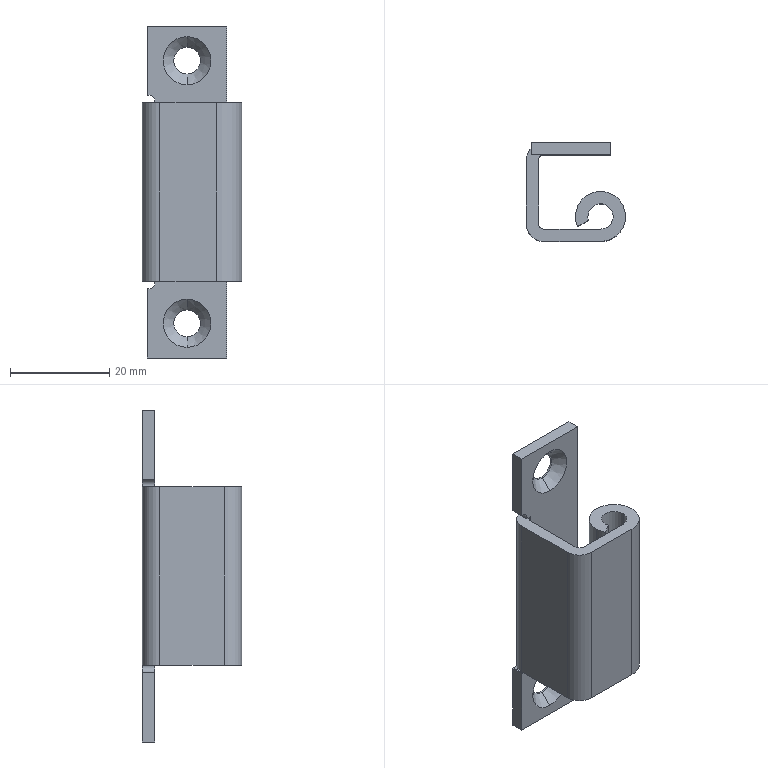Part | SolidWorks | features BaseBody 1 | 1 solid | 38 faces | box 20 x 20 x 67 mm | volume 6811 mm3 | plane 18 | cylinder 16 | cone 4 | commonest cylinder face diameters 5.4 x4 5.1 x3 10.1 x3 2 x2 2.5 x2 7 x2
STEP:
#1=CARTESIAN_POINT('',(-5.95,14.6,23.8));
#2=VERTEX_POINT('',#1);
#3=CARTESIAN_POINT('',(-5.95,14.6,29.2));
#4=VERTEX_POINT('',#3);
#5=CARTESIAN_POINT('',(-5.95,14.6,26.5));
#6=DIRECTION('',(0.,1.,0.));
#7=DIRECTION('',(0.,0.,1.));
#8=AXIS2_PLACEMENT_3D('',#5,#6,#7);
#9=CIRCLE('',#8,2.7);
#10=EDGE_CURVE('',#2,#4,#9,.T.);
#11=ORIENTED_EDGE('',*,*,#10,.F.);
#12=CARTESIAN_POINT('',(-5.95,14.95,23.8));
#13=VERTEX_POINT('',#12);
#14=CARTESIAN_POINT('',(-5.95,12.45,23.8));
#15=DIRECTION('',(0.,1.,0.));
#16=VECTOR('',#15,1000.);
#17=LINE('',#14,#16);
#18=EDGE_CURVE('',#2,#13,#17,.T.);
#19=ORIENTED_EDGE('',*,*,#18,.T.);
#20=CARTESIAN_POINT('',(-5.95,14.95,29.2));
#21=VERTEX_POINT('',#20);
#22=CARTESIAN_POINT('',(-5.95,14.95,26.5));
#23=DIRECTION('',(0.,1.,0.));
#24=DIRECTION('',(0.,0.,1.));
#25=AXIS2_PLACEMENT_3D('',#22,#23,#24);
#26=CIRCLE('',#25,2.7);
#27=EDGE_CURVE('',#13,#21,#26,.T.);
#28=ORIENTED_EDGE('',*,*,#27,.T.);
#29=CARTESIAN_POINT('',(-5.95,12.45,29.2));
#30=DIRECTION('',(0.,1.,0.));
#31=VECTOR('',#30,1000.);
#32=LINE('',#29,#31);
#33=EDGE_CURVE('',#4,#21,#32,.T.);
#34=ORIENTED_EDGE('',*,*,#33,.F.);
#35=EDGE_LOOP('',(#11,#19,#28,#34));
#36=FACE_OUTER_BOUND('',#35,.T.);
#37=CARTESIAN_POINT('',(-5.95,12.45,26.5));
#38=DIRECTION('',(0.,1.,0.));
#39=DIRECTION('',(0.,0.,1.));
#40=AXIS2_PLACEMENT_3D('',#37,#38,#39);
#41=CYLINDRICAL_SURFACE('',#40,2.7);
#42=ADVANCED_FACE('',(#36),#41,.F.);
#43=CARTESIAN_POINT('',(-5.95,14.6,-29.2));
#44=VERTEX_POINT('',#43);
#45=CARTESIAN_POINT('',(-5.95,14.6,-23.8));
#46=VERTEX_POINT('',#45);
#47=CARTESIAN_POINT('',(-5.95,14.6,-26.5));
#48=DIRECTION('',(0.,1.,0.));
#49=DIRECTION('',(0.,0.,1.));
#50=AXIS2_PLACEMENT_3D('',#47,#48,#49);
#51=CIRCLE('',#50,2.7);
#52=EDGE_CURVE('',#44,#46,#51,.T.);
#53=ORIENTED_EDGE('',*,*,#52,.F.);
#54=CARTESIAN_POINT('',(-5.95,14.95,-29.2));
#55=VERTEX_POINT('',#54);
#56=CARTESIAN_POINT('',(-5.95,12.45,-29.2));
#57=DIRECTION('',(0.,1.,0.));
#58=VECTOR('',#57,1000.);
#59=LINE('',#56,#58);
#60=EDGE_CURVE('',#44,#55,#59,.T.);
#61=ORIENTED_EDGE('',*,*,#60,.T.);
#62=CARTESIAN_POINT('',(-5.95,14.95,-23.8));
#63=VERTEX_POINT('',#62);
#64=CARTESIAN_POINT('',(-5.95,14.95,-26.5));
#65=DIRECTION('',(0.,1.,0.));
#66=DIRECTION('',(0.,0.,1.));
#67=AXIS2_PLACEMENT_3D('',#64,#65,#66);
#68=CIRCLE('',#67,2.7);
#69=EDGE_CURVE('',#55,#63,#68,.T.);
#70=ORIENTED_EDGE('',*,*,#69,.T.);
#71=CARTESIAN_POINT('',(-5.95,12.45,-23.8));
#72=DIRECTION('',(0.,1.,0.));
#73=VECTOR('',#72,1000.);
#74=LINE('',#71,#73);
#75=EDGE_CURVE('',#46,#63,#74,.T.);
#76=ORIENTED_EDGE('',*,*,#75,.F.);
#77=EDGE_LOOP('',(#53,#61,#70,#76));
#78=FACE_OUTER_BOUND('',#77,.T.);
#79=CARTESIAN_POINT('',(-5.95,12.45,-26.5));
#80=DIRECTION('',(0.,1.,0.));
#81=DIRECTION('',(0.,0.,1.));
#82=AXIS2_PLACEMENT_3D('',#79,#80,#81);
#83=CYLINDRICAL_SURFACE('',#82,2.7);
#84=ADVANCED_FACE('',(#78),#83,.F.);
#85=ORIENTED_EDGE('',*,*,#10,.T.);
#86=CARTESIAN_POINT('',(-5.95,12.45,31.35));
#87=VERTEX_POINT('',#86);
#88=CARTESIAN_POINT('',(-5.95,12.45,31.35));
#89=DIRECTION('',(0.,-0.7071,0.7071));
#90=VECTOR('',#89,1000.);
#91=LINE('',#88,#90);
#92=EDGE_CURVE('',#4,#87,#91,.T.);
#93=ORIENTED_EDGE('',*,*,#92,.T.);
#94=CARTESIAN_POINT('',(-5.95,12.45,21.65));
#95=VERTEX_POINT('',#94);
#96=CARTESIAN_POINT('',(-5.95,12.45,26.5));
#97=DIRECTION('',(0.,-1.,0.));
#98=DIRECTION('',(0.,0.,-1.));
#99=AXIS2_PLACEMENT_3D('',#96,#97,#98);
#100=CIRCLE('',#99,4.85);
#101=EDGE_CURVE('',#87,#95,#100,.T.);
#102=ORIENTED_EDGE('',*,*,#101,.T.);
#103=CARTESIAN_POINT('',(-5.95,12.45,21.65));
#104=DIRECTION('',(0.,-0.7071,-0.7071));
#105=VECTOR('',#104,1000.);
#106=LINE('',#103,#105);
#107=EDGE_CURVE('',#2,#95,#106,.T.);
#108=ORIENTED_EDGE('',*,*,#107,.F.);
#109=EDGE_LOOP('',(#85,#93,#102,#108));
#110=FACE_OUTER_BOUND('',#109,.T.);
#111=CARTESIAN_POINT('',(-5.95,12.45,26.5));
#112=DIRECTION('',(0.,-1.,0.));
#113=DIRECTION('',(0.,0.,-1.));
#114=AXIS2_PLACEMENT_3D('',#111,#112,#113);
#115=CONICAL_SURFACE('',#114,4.85,0.7854);
#116=ADVANCED_FACE('',(#110),#115,.F.);
#117=ORIENTED_EDGE('',*,*,#52,.T.);
#118=CARTESIAN_POINT('',(-5.95,12.45,-21.65));
#119=VERTEX_POINT('',#118);
#120=CARTESIAN_POINT('',(-5.95,12.45,-21.65));
#121=DIRECTION('',(0.,-0.7071,0.7071));
#122=VECTOR('',#121,1000.);
#123=LINE('',#120,#122);
#124=EDGE_CURVE('',#46,#119,#123,.T.);
#125=ORIENTED_EDGE('',*,*,#124,.T.);
#126=CARTESIAN_POINT('',(-5.95,12.45,-31.35));
#127=VERTEX_POINT('',#126);
#128=CARTESIAN_POINT('',(-5.95,12.45,-26.5));
#129=DIRECTION('',(0.,-1.,0.));
#130=DIRECTION('',(0.,0.,-1.));
#131=AXIS2_PLACEMENT_3D('',#128,#129,#130);
#132=CIRCLE('',#131,4.85);
#133=EDGE_CURVE('',#119,#127,#132,.T.);
#134=ORIENTED_EDGE('',*,*,#133,.T.);
#135=CARTESIAN_POINT('',(-5.95,12.45,-31.35));
#136=DIRECTION('',(0.,-0.7071,-0.7071));
#137=VECTOR('',#136,1000.);
#138=LINE('',#135,#137);
#139=EDGE_CURVE('',#44,#127,#138,.T.);
#140=ORIENTED_EDGE('',*,*,#139,.F.);
#141=EDGE_LOOP('',(#117,#125,#134,#140));
#142=FACE_OUTER_BOUND('',#141,.T.);
#143=CARTESIAN_POINT('',(-5.95,12.45,-26.5));
#144=DIRECTION('',(0.,-1.,0.));
#145=DIRECTION('',(0.,0.,-1.));
#146=AXIS2_PLACEMENT_3D('',#143,#144,#145);
#147=CONICAL_SURFACE('',#146,4.85,0.7854);
#148=ADVANCED_FACE('',(#142),#147,.F.);
#149=CARTESIAN_POINT('',(-2.426,-0.7856,-18.));
#150=VERTEX_POINT('',#149);
#151=CARTESIAN_POINT('',(-2.55,0.,-18.));
#152=VERTEX_POINT('',#151);
#153=CARTESIAN_POINT('',(0.,0.,-18.));
#154=DIRECTION('',(0.,0.,-1.));
#155=DIRECTION('',(1.,0.,0.));
#156=AXIS2_PLACEMENT_3D('',#153,#154,#155);
#157=CIRCLE('',#156,2.55);
#158=EDGE_CURVE('',#150,#152,#157,.T.);
#159=ORIENTED_EDGE('',*,*,#158,.T.);
#160=CARTESIAN_POINT('',(-2.55,0.,18.));
#161=VERTEX_POINT('',#160);
#162=CARTESIAN_POINT('',(-2.55,0.,18.));
#163=DIRECTION('',(0.,0.,1.));
#164=VECTOR('',#163,1000.);
#165=LINE('',#162,#164);
#166=EDGE_CURVE('',#152,#161,#165,.T.);
#167=ORIENTED_EDGE('',*,*,#166,.T.);
#168=CARTESIAN_POINT('',(-2.426,-0.7856,18.));
#169=VERTEX_POINT('',#168);
#170=CARTESIAN_POINT('',(0.,0.,18.));
#171=DIRECTION('',(0.,0.,-1.));
#172=DIRECTION('',(1.,0.,0.));
#173=AXIS2_PLACEMENT_3D('',#170,#171,#172);
#174=CIRCLE('',#173,2.55);
#175=EDGE_CURVE('',#169,#161,#174,.T.);
#176=ORIENTED_EDGE('',*,*,#175,.F.);
#177=CARTESIAN_POINT('',(-2.426,-0.7856,18.));
#178=DIRECTION('',(0.,0.,-1.));
#179=VECTOR('',#178,1000.);
#180=LINE('',#177,#179);
#181=EDGE_CURVE('',#169,#150,#180,.T.);
#182=ORIENTED_EDGE('',*,*,#181,.T.);
#183=EDGE_LOOP('',(#159,#167,#176,#182));
#184=FACE_OUTER_BOUND('',#183,.T.);
#185=CARTESIAN_POINT('',(0.,0.,18.));
#186=DIRECTION('',(0.,0.,1.));
#187=DIRECTION('',(1.,0.,0.));
#188=AXIS2_PLACEMENT_3D('',#185,#186,#187);
#189=CYLINDRICAL_SURFACE('',#188,2.55);
#190=ADVANCED_FACE('',(#184),#189,.F.);
#191=ORIENTED_EDGE('',*,*,#166,.F.);
#192=CARTESIAN_POINT('',(2.55,0.,-18.));
#193=VERTEX_POINT('',#192);
#194=CARTESIAN_POINT('',(0.,0.,-18.));
#195=DIRECTION('',(0.,0.,-1.));
#196=DIRECTION('',(1.,0.,0.));
#197=AXIS2_PLACEMENT_3D('',#194,#195,#196);
#198=CIRCLE('',#197,2.55);
#199=EDGE_CURVE('',#152,#193,#198,.T.);
#200=ORIENTED_EDGE('',*,*,#199,.T.);
#201=CARTESIAN_POINT('',(2.55,0.,18.));
#202=VERTEX_POINT('',#201);
#203=CARTESIAN_POINT('',(2.55,0.,18.));
#204=DIRECTION('',(0.,0.,1.));
#205=VECTOR('',#204,1000.);
#206=LINE('',#203,#205);
#207=EDGE_CURVE('',#193,#202,#206,.T.);
#208=ORIENTED_EDGE('',*,*,#207,.T.);
#209=CARTESIAN_POINT('',(0.,0.,18.));
#210=DIRECTION('',(0.,0.,-1.));
#211=DIRECTION('',(1.,0.,0.));
#212=AXIS2_PLACEMENT_3D('',#209,#210,#211);
#213=CIRCLE('',#212,2.55);
#214=EDGE_CURVE('',#161,#202,#213,.T.);
#215=ORIENTED_EDGE('',*,*,#214,.F.);
#216=EDGE_LOOP('',(#191,#200,#208,#215));
#217=FACE_OUTER_BOUND('',#216,.T.);
#218=CARTESIAN_POINT('',(0.,0.,18.));
#219=DIRECTION('',(0.,0.,1.));
#220=DIRECTION('',(1.,0.,0.));
#221=AXIS2_PLACEMENT_3D('',#218,#219,#220);
#222=CYLINDRICAL_SURFACE('',#221,2.55);
#223=ADVANCED_FACE('',(#217),#222,.F.);
#224=CARTESIAN_POINT('',(5.05,0.,-18.));
#225=VERTEX_POINT('',#224);
#226=CARTESIAN_POINT('',(-5.05,0.,-18.));
#227=VERTEX_POINT('',#226);
#228=CARTESIAN_POINT('',(0.,0.,-18.));
#229=DIRECTION('',(0.,0.,1.));
#230=DIRECTION('',(1.,0.,0.));
#231=AXIS2_PLACEMENT_3D('',#228,#229,#230);
#232=CIRCLE('',#231,5.05);
#233=EDGE_CURVE('',#225,#227,#232,.T.);
#234=ORIENTED_EDGE('',*,*,#233,.T.);
#235=CARTESIAN_POINT('',(-5.05,0.,18.));
#236=VERTEX_POINT('',#235);
#237=CARTESIAN_POINT('',(-5.05,0.,18.));
#238=DIRECTION('',(0.,0.,1.));
#239=VECTOR('',#238,1000.);
#240=LINE('',#237,#239);
#241=EDGE_CURVE('',#227,#236,#240,.T.);
#242=ORIENTED_EDGE('',*,*,#241,.T.);
#243=CARTESIAN_POINT('',(5.05,0.,18.));
#244=VERTEX_POINT('',#243);
#245=CARTESIAN_POINT('',(0.,0.,18.));
#246=DIRECTION('',(0.,0.,1.));
#247=DIRECTION('',(1.,0.,0.));
#248=AXIS2_PLACEMENT_3D('',#245,#246,#247);
#249=CIRCLE('',#248,5.05);
#250=EDGE_CURVE('',#244,#236,#249,.T.);
#251=ORIENTED_EDGE('',*,*,#250,.F.);
#252=CARTESIAN_POINT('',(5.05,0.,18.));
#253=DIRECTION('',(0.,0.,1.));
#254=VECTOR('',#253,1000.);
#255=LINE('',#252,#254);
#256=EDGE_CURVE('',#225,#244,#255,.T.);
#257=ORIENTED_EDGE('',*,*,#256,.F.);
#258=EDGE_LOOP('',(#234,#242,#251,#257));
#259=FACE_OUTER_BOUND('',#258,.T.);
#260=CARTESIAN_POINT('',(0.,0.,18.));
#261=DIRECTION('',(0.,0.,1.));
#262=DIRECTION('',(1.,0.,0.));
#263=AXIS2_PLACEMENT_3D('',#260,#261,#262);
#264=CYLINDRICAL_SURFACE('',#263,5.05);
#265=ADVANCED_FACE('',(#259),#264,.T.);
#266=CARTESIAN_POINT('',(0.,-5.05,-18.));
#267=VERTEX_POINT('',#266);
#268=CARTESIAN_POINT('',(0.,0.,-18.));
#269=DIRECTION('',(0.,0.,1.));
#270=DIRECTION('',(1.,0.,0.));
#271=AXIS2_PLACEMENT_3D('',#268,#269,#270);
#272=CIRCLE('',#271,5.05);
#273=EDGE_CURVE('',#267,#225,#272,.T.);
#274=ORIENTED_EDGE('',*,*,#273,.T.);
#275=ORIENTED_EDGE('',*,*,#256,.T.);
#276=CARTESIAN_POINT('',(0.,-5.05,18.));
#277=VERTEX_POINT('',#276);
#278=CARTESIAN_POINT('',(0.,0.,18.));
#279=DIRECTION('',(0.,0.,1.));
#280=DIRECTION('',(1.,0.,0.));
#281=AXIS2_PLACEMENT_3D('',#278,#279,#280);
#282=CIRCLE('',#281,5.05);
#283=EDGE_CURVE('',#277,#244,#282,.T.);
#284=ORIENTED_EDGE('',*,*,#283,.F.);
#285=CARTESIAN_POINT('',(0.,-5.05,18.));
#286=DIRECTION('',(0.,0.,-1.));
#287=VECTOR('',#286,1000.);
#288=LINE('',#285,#287);
#289=EDGE_CURVE('',#277,#267,#288,.T.);
#290=ORIENTED_EDGE('',*,*,#289,.T.);
#291=EDGE_LOOP('',(#274,#275,#284,#290));
#292=FACE_OUTER_BOUND('',#291,.T.);
#293=CARTESIAN_POINT('',(0.,0.,18.));
#294=DIRECTION('',(0.,0.,1.));
#295=DIRECTION('',(1.,0.,0.));
#296=AXIS2_PLACEMENT_3D('',#293,#294,#295);
#297=CYLINDRICAL_SURFACE('',#296,5.05);
#298=ADVANCED_FACE('',(#292),#297,.T.);
#299=CARTESIAN_POINT('',(-13.95,14.95,-33.5));
#300=VERTEX_POINT('',#299);
#301=CARTESIAN_POINT('',(2.05,14.95,-33.5));
#302=VERTEX_POINT('',#301);
#303=CARTESIAN_POINT('',(2.05,14.95,-33.5));
#304=DIRECTION('',(1.,0.,0.));
#305=VECTOR('',#304,1000.);
#306=LINE('',#303,#305);
#307=EDGE_CURVE('',#300,#302,#306,.T.);
#308=ORIENTED_EDGE('',*,*,#307,.F.);
#309=CARTESIAN_POINT('',(-13.95,14.95,-19.5));
#310=VERTEX_POINT('',#309);
#311=CARTESIAN_POINT('',(-13.95,14.95,18.));
#312=DIRECTION('',(0.,0.,-1.));
#313=VECTOR('',#312,1000.);
#314=LINE('',#311,#313);
#315=EDGE_CURVE('',#310,#300,#314,.T.);
#316=ORIENTED_EDGE('',*,*,#315,.F.);
#317=CARTESIAN_POINT('',(-13.675,14.95,-19.5));
#318=VERTEX_POINT('',#317);
#319=CARTESIAN_POINT('',(-13.95,14.95,-19.5));
#320=DIRECTION('',(-1.,0.,0.));
#321=VECTOR('',#320,1000.);
#322=LINE('',#319,#321);
#323=EDGE_CURVE('',#318,#310,#322,.T.);
#324=ORIENTED_EDGE('',*,*,#323,.F.);
#325=CARTESIAN_POINT('',(-12.45,14.95,-18.));
#326=VERTEX_POINT('',#325);
#327=CARTESIAN_POINT('',(-13.675,14.95,-18.25));
#328=DIRECTION('',(0.,1.,0.));
#329=DIRECTION('',(0.,0.,-1.));
#330=AXIS2_PLACEMENT_3D('',#327,#328,#329);
#331=CIRCLE('',#330,1.25);
#332=EDGE_CURVE('',#326,#318,#331,.T.);
#333=ORIENTED_EDGE('',*,*,#332,.F.);
#334=CARTESIAN_POINT('',(-11.45,14.95,-18.));
#335=VERTEX_POINT('',#334);
#336=CARTESIAN_POINT('',(2.05,14.95,-18.));
#337=DIRECTION('',(-1.,0.,0.));
#338=VECTOR('',#337,1000.);
#339=LINE('',#336,#338);
#340=EDGE_CURVE('',#335,#326,#339,.T.);
#341=ORIENTED_EDGE('',*,*,#340,.F.);
#342=CARTESIAN_POINT('',(-11.45,14.95,18.));
#343=VERTEX_POINT('',#342);
#344=CARTESIAN_POINT('',(-11.45,14.95,18.));
#345=DIRECTION('',(0.,0.,-1.));
#346=VECTOR('',#345,1000.);
#347=LINE('',#344,#346);
#348=EDGE_CURVE('',#343,#335,#347,.T.);
#349=ORIENTED_EDGE('',*,*,#348,.F.);
#350=CARTESIAN_POINT('',(-12.45,14.95,18.));
#351=VERTEX_POINT('',#350);
#352=CARTESIAN_POINT('',(2.05,14.95,18.));
#353=DIRECTION('',(1.,0.,0.));
#354=VECTOR('',#353,1000.);
#355=LINE('',#352,#354);
#356=EDGE_CURVE('',#351,#343,#355,.T.);
#357=ORIENTED_EDGE('',*,*,#356,.F.);
#358=CARTESIAN_POINT('',(-13.675,14.95,19.5));
#359=VERTEX_POINT('',#358);
#360=CARTESIAN_POINT('',(-13.675,14.95,18.25));
#361=DIRECTION('',(0.,1.,0.));
#362=DIRECTION('',(0.,0.,-1.));
#363=AXIS2_PLACEMENT_3D('',#360,#361,#362);
#364=CIRCLE('',#363,1.25);
#365=EDGE_CURVE('',#359,#351,#364,.T.);
#366=ORIENTED_EDGE('',*,*,#365,.F.);
#367=CARTESIAN_POINT('',(-13.95,14.95,19.5));
#368=VERTEX_POINT('',#367);
#369=CARTESIAN_POINT('',(-13.675,14.95,19.5));
#370=DIRECTION('',(1.,0.,0.));
#371=VECTOR('',#370,1000.);
#372=LINE('',#369,#371);
#373=EDGE_CURVE('',#368,#359,#372,.T.);
#374=ORIENTED_EDGE('',*,*,#373,.F.);
#375=CARTESIAN_POINT('',(-13.95,14.95,33.5));
#376=VERTEX_POINT('',#375);
#377=CARTESIAN_POINT('',(-13.95,14.95,18.));
#378=DIRECTION('',(0.,0.,-1.));
#379=VECTOR('',#378,1000.);
#380=LINE('',#377,#379);
#381=EDGE_CURVE('',#376,#368,#380,.T.);
#382=ORIENTED_EDGE('',*,*,#381,.F.);
#383=CARTESIAN_POINT('',(2.05,14.95,33.5));
#384=VERTEX_POINT('',#383);
#385=CARTESIAN_POINT('',(2.05,14.95,33.5));
#386=DIRECTION('',(-1.,0.,0.));
#387=VECTOR('',#386,1000.);
#388=LINE('',#385,#387);
#389=EDGE_CURVE('',#384,#376,#388,.T.);
#390=ORIENTED_EDGE('',*,*,#389,.F.);
#391=CARTESIAN_POINT('',(2.05,14.95,18.));
#392=DIRECTION('',(0.,0.,1.));
#393=VECTOR('',#392,1000.);
#394=LINE('',#391,#393);
#395=EDGE_CURVE('',#302,#384,#394,.T.);
#396=ORIENTED_EDGE('',*,*,#395,.F.);
#397=EDGE_LOOP('',(#308,#316,#324,#333,#341,#349,#357,#366,#374,#382,#390,#396));
#398=FACE_OUTER_BOUND('',#397,.T.);
#399=CARTESIAN_POINT('',(-5.95,14.95,26.5));
#400=DIRECTION('',(0.,1.,0.));
#401=DIRECTION('',(0.,0.,1.));
#402=AXIS2_PLACEMENT_3D('',#399,#400,#401);
#403=CIRCLE('',#402,2.7);
#404=EDGE_CURVE('',#21,#13,#403,.T.);
#405=ORIENTED_EDGE('',*,*,#404,.F.);
#406=ORIENTED_EDGE('',*,*,#27,.F.);
#407=EDGE_LOOP('',(#405,#406));
#408=FACE_BOUND('',#407,.T.);
#409=CARTESIAN_POINT('',(-5.95,14.95,-26.5));
#410=DIRECTION('',(0.,1.,0.));
#411=DIRECTION('',(0.,0.,1.));
#412=AXIS2_PLACEMENT_3D('',#409,#410,#411);
#413=CIRCLE('',#412,2.7);
#414=EDGE_CURVE('',#63,#55,#413,.T.);
#415=ORIENTED_EDGE('',*,*,#414,.F.);
#416=ORIENTED_EDGE('',*,*,#69,.F.);
#417=EDGE_LOOP('',(#415,#416));
#418=FACE_BOUND('',#417,.T.);
#419=CARTESIAN_POINT('',(2.05,14.95,18.));
#420=DIRECTION('',(0.,-1.,0.));
#421=DIRECTION('',(0.,0.,-1.));
#422=AXIS2_PLACEMENT_3D('',#419,#420,#421);
#423=PLANE('',#422);
#424=ADVANCED_FACE('',(#398,#408,#418),#423,.F.);
#425=CARTESIAN_POINT('',(2.05,12.45,-33.5));
#426=VERTEX_POINT('',#425);
#427=CARTESIAN_POINT('',(2.05,12.45,-33.5));
#428=DIRECTION('',(0.,-1.,0.));
#429=VECTOR('',#428,1000.);
#430=LINE('',#427,#429);
#431=EDGE_CURVE('',#302,#426,#430,.T.);
#432=ORIENTED_EDGE('',*,*,#431,.F.);
#433=ORIENTED_EDGE('',*,*,#395,.T.);
#434=CARTESIAN_POINT('',(2.05,12.45,33.5));
#435=VERTEX_POINT('',#434);
#436=CARTESIAN_POINT('',(2.05,12.45,33.5));
#437=DIRECTION('',(0.,1.,0.));
#438=VECTOR('',#437,1000.);
#439=LINE('',#436,#438);
#440=EDGE_CURVE('',#435,#384,#439,.T.);
#441=ORIENTED_EDGE('',*,*,#440,.F.);
#442=CARTESIAN_POINT('',(2.05,12.45,18.));
#443=DIRECTION('',(0.,0.,1.));
#444=VECTOR('',#443,1000.);
#445=LINE('',#442,#444);
#446=EDGE_CURVE('',#426,#435,#445,.T.);
#447=ORIENTED_EDGE('',*,*,#446,.F.);
#448=EDGE_LOOP('',(#432,#433,#441,#447));
#449=FACE_OUTER_BOUND('',#448,.T.);
#450=CARTESIAN_POINT('',(2.05,12.45,18.));
#451=DIRECTION('',(-1.,0.,0.));
#452=DIRECTION('',(0.,0.,1.));
#453=AXIS2_PLACEMENT_3D('',#450,#451,#452);
#454=PLANE('',#453);
#455=ADVANCED_FACE('',(#449),#454,.F.);
#456=CARTESIAN_POINT('',(-13.95,12.45,-33.5));
#457=VERTEX_POINT('',#456);
#458=CARTESIAN_POINT('',(2.05,12.45,-33.5));
#459=DIRECTION('',(-1.,0.,0.));
#460=VECTOR('',#459,1000.);
#461=LINE('',#458,#460);
#462=EDGE_CURVE('',#426,#457,#461,.T.);
#463=ORIENTED_EDGE('',*,*,#462,.T.);
#464=CARTESIAN_POINT('',(-13.95,12.45,-33.5));
#465=DIRECTION('',(0.,1.,0.));
#466=VECTOR('',#465,1000.);
#467=LINE('',#464,#466);
#468=EDGE_CURVE('',#457,#300,#467,.T.);
#469=ORIENTED_EDGE('',*,*,#468,.T.);
#470=ORIENTED_EDGE('',*,*,#307,.T.);
#471=ORIENTED_EDGE('',*,*,#431,.T.);
#472=EDGE_LOOP('',(#463,#469,#470,#471));
#473=FACE_OUTER_BOUND('',#472,.T.);
#474=CARTESIAN_POINT('',(2.05,12.45,-33.5));
#475=DIRECTION('',(0.,0.,-1.));
#476=DIRECTION('',(-1.,0.,0.));
#477=AXIS2_PLACEMENT_3D('',#474,#475,#476);
#478=PLANE('',#477);
#479=ADVANCED_FACE('',(#473),#478,.T.);
#480=CARTESIAN_POINT('',(-13.95,12.45,-19.5));
#481=VERTEX_POINT('',#480);
#482=CARTESIAN_POINT('',(-13.95,12.45,-33.5));
#483=DIRECTION('',(0.,0.,1.));
#484=VECTOR('',#483,1000.);
#485=LINE('',#482,#484);
#486=EDGE_CURVE('',#457,#481,#485,.T.);
#487=ORIENTED_EDGE('',*,*,#486,.T.);
#488=CARTESIAN_POINT('',(-13.95,12.45,-19.5));
#489=DIRECTION('',(0.,1.,0.));
#490=VECTOR('',#489,1000.);
#491=LINE('',#488,#490);
#492=EDGE_CURVE('',#481,#310,#491,.T.);
#493=ORIENTED_EDGE('',*,*,#492,.T.);
#494=ORIENTED_EDGE('',*,*,#315,.T.);
#495=ORIENTED_EDGE('',*,*,#468,.F.);
#496=EDGE_LOOP('',(#487,#493,#494,#495));
#497=FACE_OUTER_BOUND('',#496,.T.);
#498=CARTESIAN_POINT('',(-13.95,12.45,-33.5));
#499=DIRECTION('',(-1.,0.,0.));
#500=DIRECTION('',(0.,0.,1.));
#501=AXIS2_PLACEMENT_3D('',#498,#499,#500);
#502=PLANE('',#501);
#503=ADVANCED_FACE('',(#497),#502,.T.);
#504=ORIENTED_EDGE('',*,*,#332,.T.);
#505=CARTESIAN_POINT('',(-13.675,12.45,-19.5));
#506=VERTEX_POINT('',#505);
#507=CARTESIAN_POINT('',(-13.675,12.45,-19.5));
#508=DIRECTION('',(0.,1.,0.));
#509=VECTOR('',#508,1000.);
#510=LINE('',#507,#509);
#511=EDGE_CURVE('',#506,#318,#510,.T.);
#512=ORIENTED_EDGE('',*,*,#511,.F.);
#513=CARTESIAN_POINT('',(-12.45,12.45,-18.));
#514=VERTEX_POINT('',#513);
#515=CARTESIAN_POINT('',(-13.675,12.45,-18.25));
#516=DIRECTION('',(0.,1.,0.));
#517=DIRECTION('',(0.,0.,-1.));
#518=AXIS2_PLACEMENT_3D('',#515,#516,#517);
#519=CIRCLE('',#518,1.25);
#520=EDGE_CURVE('',#514,#506,#519,.T.);
#521=ORIENTED_EDGE('',*,*,#520,.F.);
#522=CARTESIAN_POINT('',(-12.45,14.804,-18.));
#523=VERTEX_POINT('',#522);
#524=CARTESIAN_POINT('',(-12.45,12.45,-18.));
#525=DIRECTION('',(0.,-1.,0.));
#526=VECTOR('',#525,1000.);
#527=LINE('',#524,#526);
#528=EDGE_CURVE('',#523,#514,#527,.T.);
#529=ORIENTED_EDGE('',*,*,#528,.F.);
#530=CARTESIAN_POINT('',(-12.45,12.45,-18.));
#531=DIRECTION('',(0.,-1.,0.));
#532=VECTOR('',#531,1000.);
#533=LINE('',#530,#532);
#534=EDGE_CURVE('',#326,#523,#533,.T.);
#535=ORIENTED_EDGE('',*,*,#534,.F.);
#536=EDGE_LOOP('',(#504,#512,#521,#529,#535));
#537=FACE_OUTER_BOUND('',#536,.T.);
#538=CARTESIAN_POINT('',(-13.675,12.45,-18.25));
#539=DIRECTION('',(0.,-1.,0.));
#540=DIRECTION('',(0.,0.,-1.));
#541=AXIS2_PLACEMENT_3D('',#538,#539,#540);
#542=CYLINDRICAL_SURFACE('',#541,1.25);
#543=ADVANCED_FACE('',(#537),#542,.F.);
#544=ORIENTED_EDGE('',*,*,#340,.T.);
#545=ORIENTED_EDGE('',*,*,#534,.T.);
#546=CARTESIAN_POINT('',(-11.45,11.45,-18.));
#547=DIRECTION('',(0.,0.,-1.));
#548=DIRECTION('',(1.,0.,0.));
#549=AXIS2_PLACEMENT_3D('',#546,#547,#548);
#550=CIRCLE('',#549,3.5);
#551=EDGE_CURVE('',#523,#335,#550,.T.);
#552=ORIENTED_EDGE('',*,*,#551,.T.);
#553=EDGE_LOOP('',(#544,#545,#552));
#554=FACE_OUTER_BOUND('',#553,.T.);
#555=CARTESIAN_POINT('',(-12.45,12.45,-18.));
#556=DIRECTION('',(0.,0.,1.));
#557=DIRECTION('',(1.,0.,0.));
#558=AXIS2_PLACEMENT_3D('',#555,#556,#557);
#559=PLANE('',#558);
#560=ADVANCED_FACE('',(#554),#559,.T.);
#561=CARTESIAN_POINT('',(-12.45,14.804,18.));
#562=VERTEX_POINT('',#561);
#563=CARTESIAN_POINT('',(-11.45,11.45,18.));
#564=DIRECTION('',(0.,0.,-1.));
#565=DIRECTION('',(1.,0.,0.));
#566=AXIS2_PLACEMENT_3D('',#563,#564,#565);
#567=CIRCLE('',#566,3.5);
#568=EDGE_CURVE('',#562,#343,#567,.T.);
#569=ORIENTED_EDGE('',*,*,#568,.T.);
#570=ORIENTED_EDGE('',*,*,#348,.T.);
#571=ORIENTED_EDGE('',*,*,#551,.F.);
#572=CARTESIAN_POINT('',(-14.95,11.45,-18.));
#573=VERTEX_POINT('',#572);
#574=CARTESIAN_POINT('',(-11.45,11.45,-18.));
#575=DIRECTION('',(0.,0.,1.));
#576=DIRECTION('',(1.,0.,0.));
#577=AXIS2_PLACEMENT_3D('',#574,#575,#576);
#578=CIRCLE('',#577,3.5);
#579=EDGE_CURVE('',#523,#573,#578,.T.);
#580=ORIENTED_EDGE('',*,*,#579,.T.);
#581=CARTESIAN_POINT('',(-14.95,11.45,18.));
#582=VERTEX_POINT('',#581);
#583=CARTESIAN_POINT('',(-14.95,11.45,18.));
#584=DIRECTION('',(0.,0.,1.));
#585=VECTOR('',#584,1000.);
#586=LINE('',#583,#585);
#587=EDGE_CURVE('',#573,#582,#586,.T.);
#588=ORIENTED_EDGE('',*,*,#587,.T.);
#589=CARTESIAN_POINT('',(-11.45,11.45,18.));
#590=DIRECTION('',(0.,0.,-1.));
#591=DIRECTION('',(1.,0.,0.));
#592=AXIS2_PLACEMENT_3D('',#589,#590,#591);
#593=CIRCLE('',#592,3.5);
#594=EDGE_CURVE('',#582,#562,#593,.T.);
#595=ORIENTED_EDGE('',*,*,#594,.T.);
#596=EDGE_LOOP('',(#569,#570,#571,#580,#588,#595));
#597=FACE_OUTER_BOUND('',#596,.T.);
#598=CARTESIAN_POINT('',(-11.45,11.45,18.));
#599=DIRECTION('',(0.,0.,1.));
#600=DIRECTION('',(1.,0.,0.));
#601=AXIS2_PLACEMENT_3D('',#598,#599,#600);
#602=CYLINDRICAL_SURFACE('',#601,3.5);
#603=ADVANCED_FACE('',(#597),#602,.T.);
#604=CARTESIAN_POINT('',(-12.45,12.45,18.));
#605=DIRECTION('',(0.,1.,0.));
#606=VECTOR('',#605,1000.);
#607=LINE('',#604,#606);
#608=EDGE_CURVE('',#562,#351,#607,.T.);
#609=ORIENTED_EDGE('',*,*,#608,.T.);
#610=ORIENTED_EDGE('',*,*,#356,.T.);
#611=ORIENTED_EDGE('',*,*,#568,.F.);
#612=EDGE_LOOP('',(#609,#610,#611));
#613=FACE_OUTER_BOUND('',#612,.T.);
#614=CARTESIAN_POINT('',(-11.45,12.45,18.));
#615=DIRECTION('',(0.,0.,-1.));
#616=DIRECTION('',(-1.,0.,0.));
#617=AXIS2_PLACEMENT_3D('',#614,#615,#616);
#618=PLANE('',#617);
#619=ADVANCED_FACE('',(#613),#618,.T.);
#620=ORIENTED_EDGE('',*,*,#365,.T.);
#621=ORIENTED_EDGE('',*,*,#608,.F.);
#622=CARTESIAN_POINT('',(-12.45,12.45,18.));
#623=VERTEX_POINT('',#622);
#624=CARTESIAN_POINT('',(-12.45,12.45,18.));
#625=DIRECTION('',(0.,1.,0.));
#626=VECTOR('',#625,1000.);
#627=LINE('',#624,#626);
#628=EDGE_CURVE('',#623,#562,#627,.T.);
#629=ORIENTED_EDGE('',*,*,#628,.F.);
#630=CARTESIAN_POINT('',(-13.675,12.45,19.5));
#631=VERTEX_POINT('',#630);
#632=CARTESIAN_POINT('',(-13.675,12.45,18.25));
#633=DIRECTION('',(0.,1.,0.));
#634=DIRECTION('',(0.,0.,-1.));
#635=AXIS2_PLACEMENT_3D('',#632,#633,#634);
#636=CIRCLE('',#635,1.25);
#637=EDGE_CURVE('',#631,#623,#636,.T.);
#638=ORIENTED_EDGE('',*,*,#637,.F.);
#639=CARTESIAN_POINT('',(-13.675,12.45,19.5));
#640=DIRECTION('',(0.,-1.,0.));
#641=VECTOR('',#640,1000.);
#642=LINE('',#639,#641);
#643=EDGE_CURVE('',#359,#631,#642,.T.);
#644=ORIENTED_EDGE('',*,*,#643,.F.);
#645=EDGE_LOOP('',(#620,#621,#629,#638,#644));
#646=FACE_OUTER_BOUND('',#645,.T.);
#647=CARTESIAN_POINT('',(-13.675,12.45,18.25));
#648=DIRECTION('',(0.,-1.,0.));
#649=DIRECTION('',(0.,0.,-1.));
#650=AXIS2_PLACEMENT_3D('',#647,#648,#649);
#651=CYLINDRICAL_SURFACE('',#650,1.25);
#652=ADVANCED_FACE('',(#646),#651,.F.);
#653=CARTESIAN_POINT('',(-13.95,12.45,19.5));
#654=VERTEX_POINT('',#653);
#655=CARTESIAN_POINT('',(-13.95,12.45,33.5));
#656=VERTEX_POINT('',#655);
#657=CARTESIAN_POINT('',(-13.95,12.45,19.5));
#658=DIRECTION('',(0.,0.,1.));
#659=VECTOR('',#658,1000.);
#660=LINE('',#657,#659);
#661=EDGE_CURVE('',#654,#656,#660,.T.);
#662=ORIENTED_EDGE('',*,*,#661,.T.);
#663=CARTESIAN_POINT('',(-13.95,12.45,33.5));
#664=DIRECTION('',(0.,1.,0.));
#665=VECTOR('',#664,1000.);
#666=LINE('',#663,#665);
#667=EDGE_CURVE('',#656,#376,#666,.T.);
#668=ORIENTED_EDGE('',*,*,#667,.T.);
#669=ORIENTED_EDGE('',*,*,#381,.T.);
#670=CARTESIAN_POINT('',(-13.95,12.45,19.5));
#671=DIRECTION('',(0.,-1.,0.));
#672=VECTOR('',#671,1000.);
#673=LINE('',#670,#672);
#674=EDGE_CURVE('',#368,#654,#673,.T.);
#675=ORIENTED_EDGE('',*,*,#674,.T.);
#676=EDGE_LOOP('',(#662,#668,#669,#675));
#677=FACE_OUTER_BOUND('',#676,.T.);
#678=CARTESIAN_POINT('',(-13.95,12.45,19.5));
#679=DIRECTION('',(-1.,0.,0.));
#680=DIRECTION('',(0.,0.,1.));
#681=AXIS2_PLACEMENT_3D('',#678,#679,#680);
#682=PLANE('',#681);
#683=ADVANCED_FACE('',(#677),#682,.T.);
#684=CARTESIAN_POINT('',(-13.95,12.45,33.5));
#685=DIRECTION('',(1.,0.,0.));
#686=VECTOR('',#685,1000.);
#687=LINE('',#684,#686);
#688=EDGE_CURVE('',#656,#435,#687,.T.);
#689=ORIENTED_EDGE('',*,*,#688,.T.);
#690=ORIENTED_EDGE('',*,*,#440,.T.);
#691=ORIENTED_EDGE('',*,*,#389,.T.);
#692=ORIENTED_EDGE('',*,*,#667,.F.);
#693=EDGE_LOOP('',(#689,#690,#691,#692));
#694=FACE_OUTER_BOUND('',#693,.T.);
#695=CARTESIAN_POINT('',(-13.95,12.45,33.5));
#696=DIRECTION('',(0.,0.,1.));
#697=DIRECTION('',(1.,0.,0.));
#698=AXIS2_PLACEMENT_3D('',#695,#696,#697);
#699=PLANE('',#698);
#700=ADVANCED_FACE('',(#694),#699,.T.);
#701=ORIENTED_EDGE('',*,*,#18,.F.);
#702=CARTESIAN_POINT('',(-5.95,14.6,26.5));
#703=DIRECTION('',(0.,1.,0.));
#704=DIRECTION('',(0.,0.,1.));
#705=AXIS2_PLACEMENT_3D('',#702,#703,#704);
#706=CIRCLE('',#705,2.7);
#707=EDGE_CURVE('',#4,#2,#706,.T.);
#708=ORIENTED_EDGE('',*,*,#707,.F.);
#709=ORIENTED_EDGE('',*,*,#33,.T.);
#710=ORIENTED_EDGE('',*,*,#404,.T.);
#711=EDGE_LOOP('',(#701,#708,#709,#710));
#712=FACE_OUTER_BOUND('',#711,.T.);
#713=CARTESIAN_POINT('',(-5.95,12.45,26.5));
#714=DIRECTION('',(0.,1.,0.));
#715=DIRECTION('',(0.,0.,1.));
#716=AXIS2_PLACEMENT_3D('',#713,#714,#715);
#717=CYLINDRICAL_SURFACE('',#716,2.7);
#718=ADVANCED_FACE('',(#712),#717,.F.);
#719=ORIENTED_EDGE('',*,*,#60,.F.);
#720=CARTESIAN_POINT('',(-5.95,14.6,-26.5));
#721=DIRECTION('',(0.,1.,0.));
#722=DIRECTION('',(0.,0.,1.));
#723=AXIS2_PLACEMENT_3D('',#720,#721,#722);
#724=CIRCLE('',#723,2.7);
#725=EDGE_CURVE('',#46,#44,#724,.T.);
#726=ORIENTED_EDGE('',*,*,#725,.F.);
#727=ORIENTED_EDGE('',*,*,#75,.T.);
#728=ORIENTED_EDGE('',*,*,#414,.T.);
#729=EDGE_LOOP('',(#719,#726,#727,#728));
#730=FACE_OUTER_BOUND('',#729,.T.);
#731=CARTESIAN_POINT('',(-5.95,12.45,-26.5));
#732=DIRECTION('',(0.,1.,0.));
#733=DIRECTION('',(0.,0.,1.));
#734=AXIS2_PLACEMENT_3D('',#731,#732,#733);
#735=CYLINDRICAL_SURFACE('',#734,2.7);
#736=ADVANCED_FACE('',(#730),#735,.F.);
#737=CARTESIAN_POINT('',(-11.45,12.45,-18.));
#738=VERTEX_POINT('',#737);
#739=CARTESIAN_POINT('',(-11.45,12.45,-18.));
#740=DIRECTION('',(1.,0.,0.));
#741=VECTOR('',#740,1000.);
#742=LINE('',#739,#741);
#743=EDGE_CURVE('',#514,#738,#742,.T.);
#744=ORIENTED_EDGE('',*,*,#743,.F.);
#745=ORIENTED_EDGE('',*,*,#520,.T.);
#746=CARTESIAN_POINT('',(-11.45,12.45,-19.5));
#747=DIRECTION('',(1.,0.,0.));
#748=VECTOR('',#747,1000.);
#749=LINE('',#746,#748);
#750=EDGE_CURVE('',#481,#506,#749,.T.);
#751=ORIENTED_EDGE('',*,*,#750,.F.);
#752=ORIENTED_EDGE('',*,*,#486,.F.);
#753=ORIENTED_EDGE('',*,*,#462,.F.);
#754=ORIENTED_EDGE('',*,*,#446,.T.);
#755=ORIENTED_EDGE('',*,*,#688,.F.);
#756=ORIENTED_EDGE('',*,*,#661,.F.);
#757=CARTESIAN_POINT('',(-11.45,12.45,19.5));
#758=DIRECTION('',(-1.,0.,0.));
#759=VECTOR('',#758,1000.);
#760=LINE('',#757,#759);
#761=EDGE_CURVE('',#631,#654,#760,.T.);
#762=ORIENTED_EDGE('',*,*,#761,.F.);
#763=ORIENTED_EDGE('',*,*,#637,.T.);
#764=CARTESIAN_POINT('',(-11.45,12.45,18.));
#765=VERTEX_POINT('',#764);
#766=CARTESIAN_POINT('',(-11.45,12.45,18.));
#767=DIRECTION('',(-1.,0.,0.));
#768=VECTOR('',#767,1000.);
#769=LINE('',#766,#768);
#770=EDGE_CURVE('',#765,#623,#769,.T.);
#771=ORIENTED_EDGE('',*,*,#770,.F.);
#772=CARTESIAN_POINT('',(-11.45,12.45,18.));
#773=DIRECTION('',(0.,0.,1.));
#774=VECTOR('',#773,1000.);
#775=LINE('',#772,#774);
#776=EDGE_CURVE('',#738,#765,#775,.T.);
#777=ORIENTED_EDGE('',*,*,#776,.F.);
#778=EDGE_LOOP('',(#744,#745,#751,#752,#753,#754,#755,#756,#762,#763,#771,#777));
#779=FACE_OUTER_BOUND('',#778,.T.);
#780=CARTESIAN_POINT('',(-5.95,12.45,26.5));
#781=DIRECTION('',(0.,-1.,0.));
#782=DIRECTION('',(0.,0.,-1.));
#783=AXIS2_PLACEMENT_3D('',#780,#781,#782);
#784=CIRCLE('',#783,4.85);
#785=EDGE_CURVE('',#95,#87,#784,.T.);
#786=ORIENTED_EDGE('',*,*,#785,.F.);
#787=ORIENTED_EDGE('',*,*,#101,.F.);
#788=EDGE_LOOP('',(#786,#787));
#789=FACE_BOUND('',#788,.T.);
#790=CARTESIAN_POINT('',(-5.95,12.45,-26.5));
#791=DIRECTION('',(0.,-1.,0.));
#792=DIRECTION('',(0.,0.,-1.));
#793=AXIS2_PLACEMENT_3D('',#790,#791,#792);
#794=CIRCLE('',#793,4.85);
#795=EDGE_CURVE('',#127,#119,#794,.T.);
#796=ORIENTED_EDGE('',*,*,#795,.F.);
#797=ORIENTED_EDGE('',*,*,#133,.F.);
#798=EDGE_LOOP('',(#796,#797));
#799=FACE_BOUND('',#798,.T.);
#800=CARTESIAN_POINT('',(-11.45,12.45,18.));
#801=DIRECTION('',(0.,1.,0.));
#802=DIRECTION('',(0.,0.,1.));
#803=AXIS2_PLACEMENT_3D('',#800,#801,#802);
#804=PLANE('',#803);
#805=ADVANCED_FACE('',(#779,#789,#799),#804,.F.);
#806=ORIENTED_EDGE('',*,*,#750,.T.);
#807=ORIENTED_EDGE('',*,*,#511,.T.);
#808=ORIENTED_EDGE('',*,*,#323,.T.);
#809=ORIENTED_EDGE('',*,*,#492,.F.);
#810=EDGE_LOOP('',(#806,#807,#808,#809));
#811=FACE_OUTER_BOUND('',#810,.T.);
#812=CARTESIAN_POINT('',(-13.95,12.45,-19.5));
#813=DIRECTION('',(0.,0.,1.));
#814=DIRECTION('',(1.,0.,0.));
#815=AXIS2_PLACEMENT_3D('',#812,#813,#814);
#816=PLANE('',#815);
#817=ADVANCED_FACE('',(#811),#816,.T.);
#818=ORIENTED_EDGE('',*,*,#743,.T.);
#819=CARTESIAN_POINT('',(-12.45,11.45,-18.));
#820=VERTEX_POINT('',#819);
#821=CARTESIAN_POINT('',(-11.45,11.45,-18.));
#822=DIRECTION('',(0.,0.,-1.));
#823=DIRECTION('',(1.,0.,0.));
#824=AXIS2_PLACEMENT_3D('',#821,#822,#823);
#825=CIRCLE('',#824,1.);
#826=EDGE_CURVE('',#820,#738,#825,.T.);
#827=ORIENTED_EDGE('',*,*,#826,.F.);
#828=CARTESIAN_POINT('',(-12.45,-1.55,-18.));
#829=VERTEX_POINT('',#828);
#830=CARTESIAN_POINT('',(-12.45,11.45,-18.));
#831=DIRECTION('',(0.,1.,0.));
#832=VECTOR('',#831,1000.);
#833=LINE('',#830,#832);
#834=EDGE_CURVE('',#829,#820,#833,.T.);
#835=ORIENTED_EDGE('',*,*,#834,.F.);
#836=CARTESIAN_POINT('',(-11.45,-2.55,-18.));
#837=VERTEX_POINT('',#836);
#838=CARTESIAN_POINT('',(-11.45,-1.55,-18.));
#839=DIRECTION('',(0.,0.,1.));
#840=DIRECTION('',(1.,0.,0.));
#841=AXIS2_PLACEMENT_3D('',#838,#839,#840);
#842=CIRCLE('',#841,1.);
#843=EDGE_CURVE('',#829,#837,#842,.T.);
#844=ORIENTED_EDGE('',*,*,#843,.T.);
#845=CARTESIAN_POINT('',(0.,-2.55,-18.));
#846=VERTEX_POINT('',#845);
#847=CARTESIAN_POINT('',(-11.45,-2.55,-18.));
#848=DIRECTION('',(-1.,0.,0.));
#849=VECTOR('',#848,1000.);
#850=LINE('',#847,#849);
#851=EDGE_CURVE('',#846,#837,#850,.T.);
#852=ORIENTED_EDGE('',*,*,#851,.F.);
#853=CARTESIAN_POINT('',(0.,0.,-18.));
#854=DIRECTION('',(0.,0.,-1.));
#855=DIRECTION('',(1.,0.,0.));
#856=AXIS2_PLACEMENT_3D('',#853,#854,#855);
#857=CIRCLE('',#856,2.55);
#858=EDGE_CURVE('',#193,#846,#857,.T.);
#859=ORIENTED_EDGE('',*,*,#858,.F.);
#860=ORIENTED_EDGE('',*,*,#199,.F.);
#861=ORIENTED_EDGE('',*,*,#158,.F.);
#862=CARTESIAN_POINT('',(-4.615,-2.05,-18.));
#863=VERTEX_POINT('',#862);
#864=CARTESIAN_POINT('',(-4.615,-2.05,-18.));
#865=DIRECTION('',(0.866,0.5,0.));
#866=VECTOR('',#865,1000.);
#867=LINE('',#864,#866);
#868=EDGE_CURVE('',#863,#150,#867,.T.);
#869=ORIENTED_EDGE('',*,*,#868,.F.);
#870=CARTESIAN_POINT('',(0.,0.,-18.));
#871=DIRECTION('',(0.,0.,1.));
#872=DIRECTION('',(1.,0.,0.));
#873=AXIS2_PLACEMENT_3D('',#870,#871,#872);
#874=CIRCLE('',#873,5.05);
#875=EDGE_CURVE('',#227,#863,#874,.T.);
#876=ORIENTED_EDGE('',*,*,#875,.F.);
#877=ORIENTED_EDGE('',*,*,#233,.F.);
#878=ORIENTED_EDGE('',*,*,#273,.F.);
#879=CARTESIAN_POINT('',(-11.45,-5.05,-18.));
#880=VERTEX_POINT('',#879);
#881=CARTESIAN_POINT('',(-11.45,-5.05,-18.));
#882=DIRECTION('',(1.,0.,0.));
#883=VECTOR('',#882,1000.);
#884=LINE('',#881,#883);
#885=EDGE_CURVE('',#880,#267,#884,.T.);
#886=ORIENTED_EDGE('',*,*,#885,.F.);
#887=CARTESIAN_POINT('',(-14.95,-1.55,-18.));
#888=VERTEX_POINT('',#887);
#889=CARTESIAN_POINT('',(-11.45,-1.55,-18.));
#890=DIRECTION('',(0.,0.,1.));
#891=DIRECTION('',(1.,0.,0.));
#892=AXIS2_PLACEMENT_3D('',#889,#890,#891);
#893=CIRCLE('',#892,3.5);
#894=EDGE_CURVE('',#888,#880,#893,.T.);
#895=ORIENTED_EDGE('',*,*,#894,.F.);
#896=CARTESIAN_POINT('',(-14.95,11.45,-18.));
#897=DIRECTION('',(0.,-1.,0.));
#898=VECTOR('',#897,1000.);
#899=LINE('',#896,#898);
#900=EDGE_CURVE('',#573,#888,#899,.T.);
#901=ORIENTED_EDGE('',*,*,#900,.F.);
#902=ORIENTED_EDGE('',*,*,#579,.F.);
#903=ORIENTED_EDGE('',*,*,#528,.T.);
#904=EDGE_LOOP('',(#818,#827,#835,#844,#852,#859,#860,#861,#869,#876,#877,#878,#886,#895,#901,#902,#903));
#905=FACE_OUTER_BOUND('',#904,.T.);
#906=CARTESIAN_POINT('',(-11.45,11.45,-18.));
#907=DIRECTION('',(0.,0.,1.));
#908=DIRECTION('',(1.,0.,0.));
#909=AXIS2_PLACEMENT_3D('',#906,#907,#908);
#910=PLANE('',#909);
#911=ADVANCED_FACE('',(#905),#910,.F.);
#912=CARTESIAN_POINT('',(-12.45,-1.55,18.));
#913=VERTEX_POINT('',#912);
#914=CARTESIAN_POINT('',(-12.45,11.45,18.));
#915=VERTEX_POINT('',#914);
#916=CARTESIAN_POINT('',(-12.45,11.45,18.));
#917=DIRECTION('',(0.,1.,0.));
#918=VECTOR('',#917,1000.);
#919=LINE('',#916,#918);
#920=EDGE_CURVE('',#913,#915,#919,.T.);
#921=ORIENTED_EDGE('',*,*,#920,.T.);
#922=CARTESIAN_POINT('',(-11.45,11.45,18.));
#923=DIRECTION('',(0.,0.,-1.));
#924=DIRECTION('',(1.,0.,0.));
#925=AXIS2_PLACEMENT_3D('',#922,#923,#924);
#926=CIRCLE('',#925,1.);
#927=EDGE_CURVE('',#915,#765,#926,.T.);
#928=ORIENTED_EDGE('',*,*,#927,.T.);
#929=ORIENTED_EDGE('',*,*,#770,.T.);
#930=ORIENTED_EDGE('',*,*,#628,.T.);
#931=ORIENTED_EDGE('',*,*,#594,.F.);
#932=CARTESIAN_POINT('',(-14.95,-1.55,18.));
#933=VERTEX_POINT('',#932);
#934=CARTESIAN_POINT('',(-14.95,11.45,18.));
#935=DIRECTION('',(0.,-1.,0.));
#936=VECTOR('',#935,1000.);
#937=LINE('',#934,#936);
#938=EDGE_CURVE('',#582,#933,#937,.T.);
#939=ORIENTED_EDGE('',*,*,#938,.T.);
#940=CARTESIAN_POINT('',(-11.45,-5.05,18.));
#941=VERTEX_POINT('',#940);
#942=CARTESIAN_POINT('',(-11.45,-1.55,18.));
#943=DIRECTION('',(0.,0.,1.));
#944=DIRECTION('',(1.,0.,0.));
#945=AXIS2_PLACEMENT_3D('',#942,#943,#944);
#946=CIRCLE('',#945,3.5);
#947=EDGE_CURVE('',#933,#941,#946,.T.);
#948=ORIENTED_EDGE('',*,*,#947,.T.);
#949=CARTESIAN_POINT('',(-11.45,-5.05,18.));
#950=DIRECTION('',(1.,0.,0.));
#951=VECTOR('',#950,1000.);
#952=LINE('',#949,#951);
#953=EDGE_CURVE('',#941,#277,#952,.T.);
#954=ORIENTED_EDGE('',*,*,#953,.T.);
#955=ORIENTED_EDGE('',*,*,#283,.T.);
#956=ORIENTED_EDGE('',*,*,#250,.T.);
#957=CARTESIAN_POINT('',(-4.615,-2.05,18.));
#958=VERTEX_POINT('',#957);
#959=CARTESIAN_POINT('',(0.,0.,18.));
#960=DIRECTION('',(0.,0.,1.));
#961=DIRECTION('',(1.,0.,0.));
#962=AXIS2_PLACEMENT_3D('',#959,#960,#961);
#963=CIRCLE('',#962,5.05);
#964=EDGE_CURVE('',#236,#958,#963,.T.);
#965=ORIENTED_EDGE('',*,*,#964,.T.);
#966=CARTESIAN_POINT('',(-4.615,-2.05,18.));
#967=DIRECTION('',(0.866,0.5,0.));
#968=VECTOR('',#967,1000.);
#969=LINE('',#966,#968);
#970=EDGE_CURVE('',#958,#169,#969,.T.);
#971=ORIENTED_EDGE('',*,*,#970,.T.);
#972=ORIENTED_EDGE('',*,*,#175,.T.);
#973=ORIENTED_EDGE('',*,*,#214,.T.);
#974=CARTESIAN_POINT('',(0.,-2.55,18.));
#975=VERTEX_POINT('',#974);
#976=CARTESIAN_POINT('',(0.,0.,18.));
#977=DIRECTION('',(0.,0.,-1.));
#978=DIRECTION('',(1.,0.,0.));
#979=AXIS2_PLACEMENT_3D('',#976,#977,#978);
#980=CIRCLE('',#979,2.55);
#981=EDGE_CURVE('',#202,#975,#980,.T.);
#982=ORIENTED_EDGE('',*,*,#981,.T.);
#983=CARTESIAN_POINT('',(-11.45,-2.55,18.));
#984=VERTEX_POINT('',#983);
#985=CARTESIAN_POINT('',(-11.45,-2.55,18.));
#986=DIRECTION('',(-1.,0.,0.));
#987=VECTOR('',#986,1000.);
#988=LINE('',#985,#987);
#989=EDGE_CURVE('',#975,#984,#988,.T.);
#990=ORIENTED_EDGE('',*,*,#989,.T.);
#991=CARTESIAN_POINT('',(-11.45,-1.55,18.));
#992=DIRECTION('',(0.,0.,-1.));
#993=DIRECTION('',(1.,0.,0.));
#994=AXIS2_PLACEMENT_3D('',#991,#992,#993);
#995=CIRCLE('',#994,1.);
#996=EDGE_CURVE('',#984,#913,#995,.T.);
#997=ORIENTED_EDGE('',*,*,#996,.T.);
#998=EDGE_LOOP('',(#921,#928,#929,#930,#931,#939,#948,#954,#955,#956,#965,#971,#972,#973,#982,#990,#997));
#999=FACE_OUTER_BOUND('',#998,.T.);
#1000=CARTESIAN_POINT('',(-11.45,11.45,18.));
#1001=DIRECTION('',(0.,0.,1.));
#1002=DIRECTION('',(1.,0.,0.));
#1003=AXIS2_PLACEMENT_3D('',#1000,#1001,#1002);
#1004=PLANE('',#1003);
#1005=ADVANCED_FACE('',(#999),#1004,.T.);
#1006=CARTESIAN_POINT('',(-14.95,-1.55,18.));
#1007=DIRECTION('',(0.,0.,-1.));
#1008=VECTOR('',#1007,1000.);
#1009=LINE('',#1006,#1008);
#1010=EDGE_CURVE('',#933,#888,#1009,.T.);
#1011=ORIENTED_EDGE('',*,*,#1010,.F.);
#1012=ORIENTED_EDGE('',*,*,#938,.F.);
#1013=ORIENTED_EDGE('',*,*,#587,.F.);
#1014=ORIENTED_EDGE('',*,*,#900,.T.);
#1015=EDGE_LOOP('',(#1011,#1012,#1013,#1014));
#1016=FACE_OUTER_BOUND('',#1015,.T.);
#1017=CARTESIAN_POINT('',(-14.95,11.45,18.));
#1018=DIRECTION('',(1.,0.,0.));
#1019=DIRECTION('',(0.,0.,-1.));
#1020=AXIS2_PLACEMENT_3D('',#1017,#1018,#1019);
#1021=PLANE('',#1020);
#1022=ADVANCED_FACE('',(#1016),#1021,.F.);
#1023=ORIENTED_EDGE('',*,*,#761,.T.);
#1024=ORIENTED_EDGE('',*,*,#674,.F.);
#1025=ORIENTED_EDGE('',*,*,#373,.T.);
#1026=ORIENTED_EDGE('',*,*,#643,.T.);
#1027=EDGE_LOOP('',(#1023,#1024,#1025,#1026));
#1028=FACE_OUTER_BOUND('',#1027,.T.);
#1029=CARTESIAN_POINT('',(-13.675,12.45,19.5));
#1030=DIRECTION('',(0.,0.,-1.));
#1031=DIRECTION('',(-1.,0.,0.));
#1032=AXIS2_PLACEMENT_3D('',#1029,#1030,#1031);
#1033=PLANE('',#1032);
#1034=ADVANCED_FACE('',(#1028),#1033,.T.);
#1035=ORIENTED_EDGE('',*,*,#92,.F.);
#1036=ORIENTED_EDGE('',*,*,#707,.T.);
#1037=ORIENTED_EDGE('',*,*,#107,.T.);
#1038=ORIENTED_EDGE('',*,*,#785,.T.);
#1039=EDGE_LOOP('',(#1035,#1036,#1037,#1038));
#1040=FACE_OUTER_BOUND('',#1039,.T.);
#1041=CARTESIAN_POINT('',(-5.95,12.45,26.5));
#1042=DIRECTION('',(0.,-1.,0.));
#1043=DIRECTION('',(0.,0.,-1.));
#1044=AXIS2_PLACEMENT_3D('',#1041,#1042,#1043);
#1045=CONICAL_SURFACE('',#1044,4.85,0.7854);
#1046=ADVANCED_FACE('',(#1040),#1045,.F.);
#1047=ORIENTED_EDGE('',*,*,#124,.F.);
#1048=ORIENTED_EDGE('',*,*,#725,.T.);
#1049=ORIENTED_EDGE('',*,*,#139,.T.);
#1050=ORIENTED_EDGE('',*,*,#795,.T.);
#1051=EDGE_LOOP('',(#1047,#1048,#1049,#1050));
#1052=FACE_OUTER_BOUND('',#1051,.T.);
#1053=CARTESIAN_POINT('',(-5.95,12.45,-26.5));
#1054=DIRECTION('',(0.,-1.,0.));
#1055=DIRECTION('',(0.,0.,-1.));
#1056=AXIS2_PLACEMENT_3D('',#1053,#1054,#1055);
#1057=CONICAL_SURFACE('',#1056,4.85,0.7854);
#1058=ADVANCED_FACE('',(#1052),#1057,.F.);
#1059=ORIENTED_EDGE('',*,*,#826,.T.);
#1060=ORIENTED_EDGE('',*,*,#776,.T.);
#1061=ORIENTED_EDGE('',*,*,#927,.F.);
#1062=CARTESIAN_POINT('',(-12.45,11.45,18.));
#1063=DIRECTION('',(0.,0.,1.));
#1064=VECTOR('',#1063,1000.);
#1065=LINE('',#1062,#1064);
#1066=EDGE_CURVE('',#820,#915,#1065,.T.);
#1067=ORIENTED_EDGE('',*,*,#1066,.F.);
#1068=EDGE_LOOP('',(#1059,#1060,#1061,#1067));
#1069=FACE_OUTER_BOUND('',#1068,.T.);
#1070=CARTESIAN_POINT('',(-11.45,11.45,18.));
#1071=DIRECTION('',(0.,0.,1.));
#1072=DIRECTION('',(1.,0.,0.));
#1073=AXIS2_PLACEMENT_3D('',#1070,#1071,#1072);
#1074=CYLINDRICAL_SURFACE('',#1073,1.);
#1075=ADVANCED_FACE('',(#1069),#1074,.F.);
#1076=ORIENTED_EDGE('',*,*,#1066,.T.);
#1077=ORIENTED_EDGE('',*,*,#920,.F.);
#1078=CARTESIAN_POINT('',(-12.45,-1.55,18.));
#1079=DIRECTION('',(0.,0.,1.));
#1080=VECTOR('',#1079,1000.);
#1081=LINE('',#1078,#1080);
#1082=EDGE_CURVE('',#829,#913,#1081,.T.);
#1083=ORIENTED_EDGE('',*,*,#1082,.F.);
#1084=ORIENTED_EDGE('',*,*,#834,.T.);
#1085=EDGE_LOOP('',(#1076,#1077,#1083,#1084));
#1086=FACE_OUTER_BOUND('',#1085,.T.);
#1087=CARTESIAN_POINT('',(-12.45,-1.55,18.));
#1088=DIRECTION('',(-1.,0.,0.));
#1089=DIRECTION('',(0.,0.,1.));
#1090=AXIS2_PLACEMENT_3D('',#1087,#1088,#1089);
#1091=PLANE('',#1090);
#1092=ADVANCED_FACE('',(#1086),#1091,.F.);
#1093=CARTESIAN_POINT('',(-11.45,-2.55,18.));
#1094=DIRECTION('',(0.,0.,-1.));
#1095=VECTOR('',#1094,1000.);
#1096=LINE('',#1093,#1095);
#1097=EDGE_CURVE('',#984,#837,#1096,.T.);
#1098=ORIENTED_EDGE('',*,*,#1097,.F.);
#1099=ORIENTED_EDGE('',*,*,#989,.F.);
#1100=CARTESIAN_POINT('',(0.,-2.55,18.));
#1101=DIRECTION('',(0.,0.,1.));
#1102=VECTOR('',#1101,1000.);
#1103=LINE('',#1100,#1102);
#1104=EDGE_CURVE('',#846,#975,#1103,.T.);
#1105=ORIENTED_EDGE('',*,*,#1104,.F.);
#1106=ORIENTED_EDGE('',*,*,#851,.T.);
#1107=EDGE_LOOP('',(#1098,#1099,#1105,#1106));
#1108=FACE_OUTER_BOUND('',#1107,.T.);
#1109=CARTESIAN_POINT('',(0.,-2.55,18.));
#1110=DIRECTION('',(0.,-1.,0.));
#1111=DIRECTION('',(0.,0.,-1.));
#1112=AXIS2_PLACEMENT_3D('',#1109,#1110,#1111);
#1113=PLANE('',#1112);
#1114=ADVANCED_FACE('',(#1108),#1113,.F.);
#1115=ORIENTED_EDGE('',*,*,#207,.F.);
#1116=ORIENTED_EDGE('',*,*,#858,.T.);
#1117=ORIENTED_EDGE('',*,*,#1104,.T.);
#1118=ORIENTED_EDGE('',*,*,#981,.F.);
#1119=EDGE_LOOP('',(#1115,#1116,#1117,#1118));
#1120=FACE_OUTER_BOUND('',#1119,.T.);
#1121=CARTESIAN_POINT('',(0.,0.,18.));
#1122=DIRECTION('',(0.,0.,1.));
#1123=DIRECTION('',(1.,0.,0.));
#1124=AXIS2_PLACEMENT_3D('',#1121,#1122,#1123);
#1125=CYLINDRICAL_SURFACE('',#1124,2.55);
#1126=ADVANCED_FACE('',(#1120),#1125,.F.);
#1127=ORIENTED_EDGE('',*,*,#181,.F.);
#1128=ORIENTED_EDGE('',*,*,#970,.F.);
#1129=CARTESIAN_POINT('',(-4.615,-2.05,18.));
#1130=DIRECTION('',(0.,0.,1.));
#1131=VECTOR('',#1130,1000.);
#1132=LINE('',#1129,#1131);
#1133=EDGE_CURVE('',#863,#958,#1132,.T.);
#1134=ORIENTED_EDGE('',*,*,#1133,.F.);
#1135=ORIENTED_EDGE('',*,*,#868,.T.);
#1136=EDGE_LOOP('',(#1127,#1128,#1134,#1135));
#1137=FACE_OUTER_BOUND('',#1136,.T.);
#1138=CARTESIAN_POINT('',(-4.615,-2.05,18.));
#1139=DIRECTION('',(-0.5,0.866,0.));
#1140=DIRECTION('',(-0.866,-0.5,0.));
#1141=AXIS2_PLACEMENT_3D('',#1138,#1139,#1140);
#1142=PLANE('',#1141);
#1143=ADVANCED_FACE('',(#1137),#1142,.F.);
#1144=ORIENTED_EDGE('',*,*,#241,.F.);
#1145=ORIENTED_EDGE('',*,*,#875,.T.);
#1146=ORIENTED_EDGE('',*,*,#1133,.T.);
#1147=ORIENTED_EDGE('',*,*,#964,.F.);
#1148=EDGE_LOOP('',(#1144,#1145,#1146,#1147));
#1149=FACE_OUTER_BOUND('',#1148,.T.);
#1150=CARTESIAN_POINT('',(0.,0.,18.));
#1151=DIRECTION('',(0.,0.,1.));
#1152=DIRECTION('',(1.,0.,0.));
#1153=AXIS2_PLACEMENT_3D('',#1150,#1151,#1152);
#1154=CYLINDRICAL_SURFACE('',#1153,5.05);
#1155=ADVANCED_FACE('',(#1149),#1154,.T.);
#1156=ORIENTED_EDGE('',*,*,#289,.F.);
#1157=ORIENTED_EDGE('',*,*,#953,.F.);
#1158=CARTESIAN_POINT('',(-11.45,-5.05,18.));
#1159=DIRECTION('',(0.,0.,1.));
#1160=VECTOR('',#1159,1000.);
#1161=LINE('',#1158,#1160);
#1162=EDGE_CURVE('',#880,#941,#1161,.T.);
#1163=ORIENTED_EDGE('',*,*,#1162,.F.);
#1164=ORIENTED_EDGE('',*,*,#885,.T.);
#1165=EDGE_LOOP('',(#1156,#1157,#1163,#1164));
#1166=FACE_OUTER_BOUND('',#1165,.T.);
#1167=CARTESIAN_POINT('',(-11.45,-5.05,18.));
#1168=DIRECTION('',(0.,1.,0.));
#1169=DIRECTION('',(0.,0.,1.));
#1170=AXIS2_PLACEMENT_3D('',#1167,#1168,#1169);
#1171=PLANE('',#1170);
#1172=ADVANCED_FACE('',(#1166),#1171,.F.);
#1173=ORIENTED_EDGE('',*,*,#947,.F.);
#1174=ORIENTED_EDGE('',*,*,#1010,.T.);
#1175=ORIENTED_EDGE('',*,*,#894,.T.);
#1176=ORIENTED_EDGE('',*,*,#1162,.T.);
#1177=EDGE_LOOP('',(#1173,#1174,#1175,#1176));
#1178=FACE_OUTER_BOUND('',#1177,.T.);
#1179=CARTESIAN_POINT('',(-11.45,-1.55,18.));
#1180=DIRECTION('',(0.,0.,1.));
#1181=DIRECTION('',(1.,0.,0.));
#1182=AXIS2_PLACEMENT_3D('',#1179,#1180,#1181);
#1183=CYLINDRICAL_SURFACE('',#1182,3.5);
#1184=ADVANCED_FACE('',(#1178),#1183,.T.);
#1185=ORIENTED_EDGE('',*,*,#843,.F.);
#1186=ORIENTED_EDGE('',*,*,#1082,.T.);
#1187=ORIENTED_EDGE('',*,*,#996,.F.);
#1188=ORIENTED_EDGE('',*,*,#1097,.T.);
#1189=EDGE_LOOP('',(#1185,#1186,#1187,#1188));
#1190=FACE_OUTER_BOUND('',#1189,.T.);
#1191=CARTESIAN_POINT('',(-11.45,-1.55,18.));
#1192=DIRECTION('',(0.,0.,1.));
#1193=DIRECTION('',(1.,0.,0.));
#1194=AXIS2_PLACEMENT_3D('',#1191,#1192,#1193);
#1195=CYLINDRICAL_SURFACE('',#1194,1.);
#1196=ADVANCED_FACE('',(#1190),#1195,.F.);
#1197=CLOSED_SHELL('',(#42,#84,#116,#148,#190,#223,#265,#298,#424,#455,#479,#503,#543,#560,#603,#619,#652,#683,#700,#718,#736,#805,#817,#911,#1005,#1022,#1034,#1046,#1058,#1075,#1092,#1114,#1126,#1143,#1155,#1172,#1184,#1196));
#1198=MANIFOLD_SOLID_BREP('',#1197);
#1199=CARTESIAN_POINT('',(0.,0.,0.));
#1200=DIRECTION('',(0.,0.,1.));
#1201=DIRECTION('',(1.,0.,0.));
#1202=AXIS2_PLACEMENT_3D('',#1199,#1200,#1201);
#1203=(LENGTH_UNIT()NAMED_UNIT(*)SI_UNIT(.MILLI.,.METRE.));
#1204=UNCERTAINTY_MEASURE_WITH_UNIT(LENGTH_MEASURE(0.00001),#1203,'','');
#1205=(NAMED_UNIT(*)PLANE_ANGLE_UNIT()SI_UNIT($,.RADIAN.));
#1206=(NAMED_UNIT(*)SI_UNIT($,.STERADIAN.)SOLID_ANGLE_UNIT());
#1207=(GEOMETRIC_REPRESENTATION_CONTEXT(3)GLOBAL_UNCERTAINTY_ASSIGNED_CONTEXT((#1204))GLOBAL_UNIT_ASSIGNED_CONTEXT((#1203,#1205,#1206))REPRESENTATION_CONTEXT('',''));
#1208=ADVANCED_BREP_SHAPE_REPRESENTATION('',(#1198,#1202),#1207);